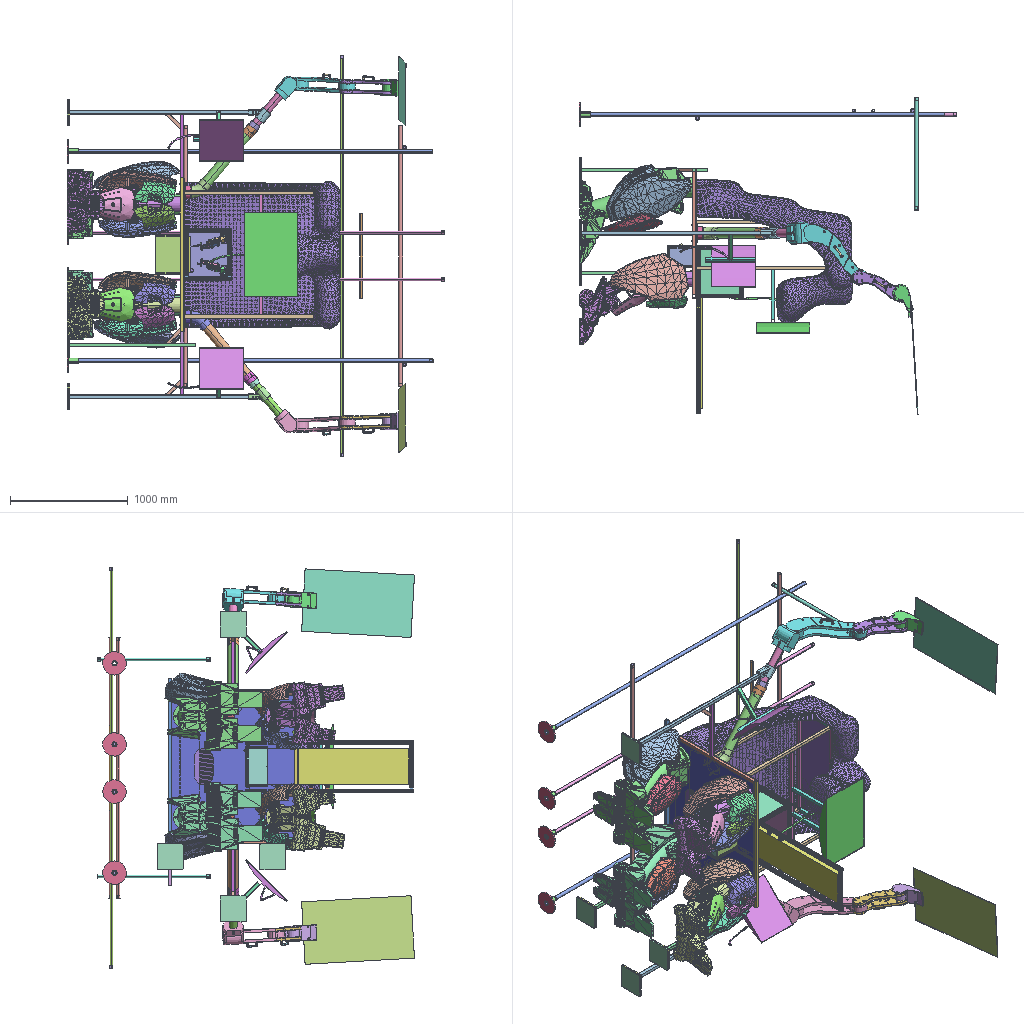Assembly | SolidWorks | 142 different items | 245 placed | box 3202 x 2687 x 3404 mm
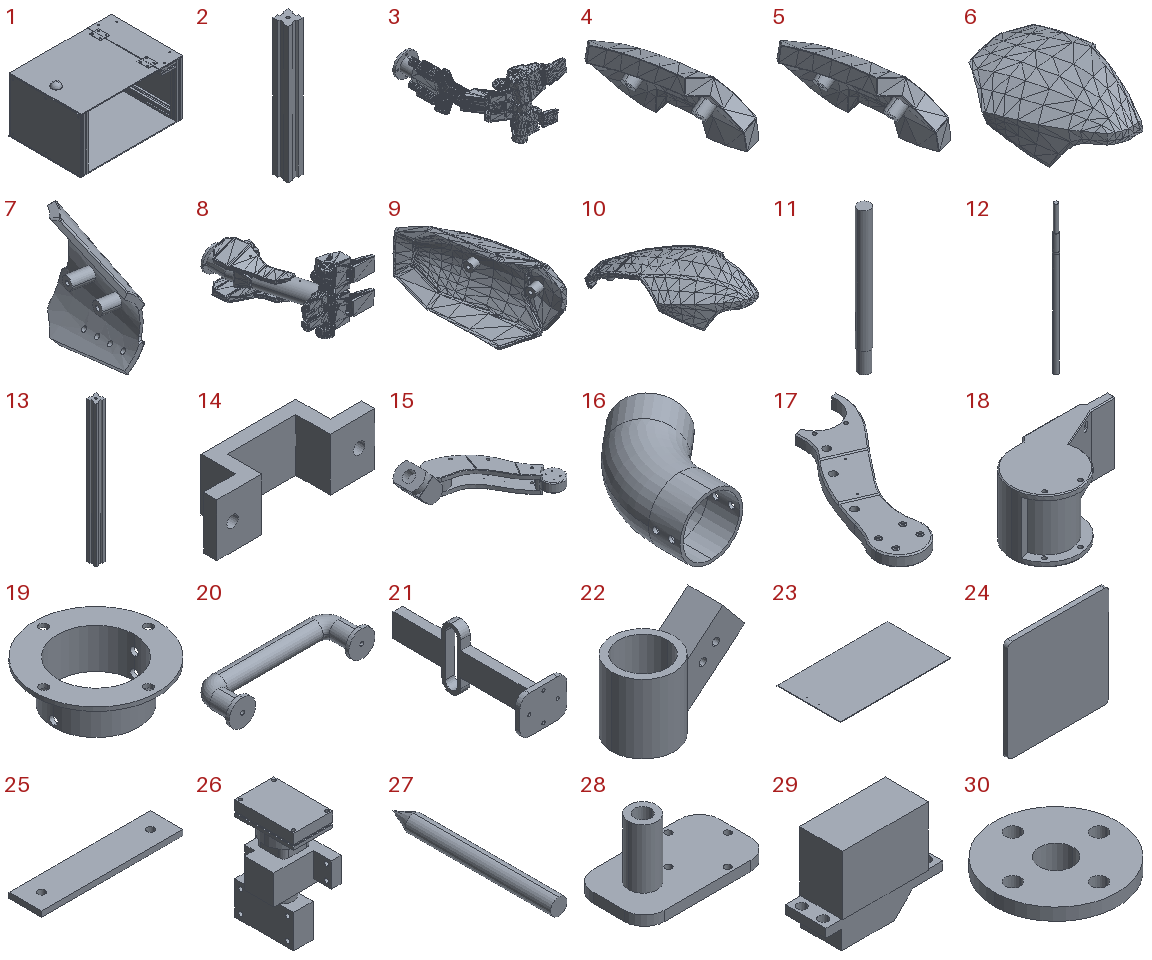Parts list (item | name | quantity | parent item | size | volume | features):
1 | (subassembly) | x1 | - | 346 x 245 x 203 mm | 1584731 mm3 | features CompositeCurve 1
2 | - | x4 | in 1 | 20 x 20 x 180 mm | 60635 mm3 | features CirPattern 1, Extrusion 1, ICE 1
3 | - | x1 | - | - | 34150920 mm3 | features MirrorStock 1
4 | - | x1 | - | 143.42 x 346.686 x 193.978 mm | 2031245 mm3 | features MirrorStock 1
5 | - | x1 | - | 143.42 x 346.686 x 193.978 mm | 2031245 mm3 | features MirrorStock 1
6 | - | x1 | - | 402.328 x 659.123 x 278.681 mm | 8547587 mm3 | features MirrorStock 1
7 | - | x1 | - | 138.848 x 288 x 292.377 mm | 1252657 mm3 | features MirrorStock 1
8 | - | x1 | - | - | 59999692 mm3 | features MirrorStock 1
9 | - | x1 | - | 192.975 x 474.444 x 296.209 mm | 2534423 mm3 | features MirrorStock 1
10 | - | x1 | - | 464.837 x 729.145 x 237.064 mm | 8192368 mm3 | features MirrorStock 1
11 | - | x1 | - | 12 x 12 x 140 mm | 15472 mm3 | features MirrorStock 1
12 | - | x1 | - | 16 x 16 x 460 mm | 67780 mm3 | features MirrorStock 1
13 | - | x1 | in 1 | 20 x 20 x 300 mm | 101058 mm3 | features CirPattern 1, Extrusion 1, ICE 1
14 | - | x1 | - | 60 x 18 x 20 mm | 8448 mm3 | features MirrorStock 1
15 | - | x1 | - | 657.517 x 555 x 192.791 mm | 7755775 mm3 | features MirrorStock 1
16 | - | x1 | - | 167.236 x 220.793 x 100 mm | 316350 mm3 | features MirrorStock 1
17 | - | x2 | - | 271.568 x 416.057 x 25 mm | 864858 mm3 | features MirrorStock 1
18 | - | x1 | - | 270 x 150 x 130 mm | 2349821 mm3 | features MirrorStock 1
19 | - | x1 | - | 160 x 160 x 52 mm | 135135 mm3 | features MirrorStock 1
20 | - | x2 | - | 122 x 37.5 x 22 mm | 26841 mm3 | features MirrorStock 1
21 | - | x1 | - | 50 x 155 x 65 mm | 47254 mm3 | features MirrorStock 1
22 | - | x1 | - | 167.949 x 90.5 x 129.102 mm | 386069 mm3 | features MirrorStock 1
23 | - | x1 | - | 930 x 530 x 5 mm | 2464158 mm3 | features MirrorStock 1
24 | - | x4 | - | 220 x 10 x 220 mm | 483142 mm3 | features Extrusion 1, Fillet 1
25 | - | x1 | - | 130 x 30 x 5 mm | 19158 mm3 | features MirrorStock 1
26 | - | x1 | - | 50 x 78.682 x 114 mm | 167439 mm3 | features MirrorStock 1
27 | - | x1 | - | 8 x 80 x 8 mm | 3686 mm3 | features MirrorStock 1
28 | - | x1 | - | 64 x 36 x 35 mm | 14420 mm3 | features MirrorStock 1
29 | - | x1 | - | 54.44 x 20 x 46.45 mm | 31100 mm3 | features MirrorStock 1
30 | - | x1 | - | 20 x 20 x 4.5 mm | 639.904 mm3 | features MirrorStock 1
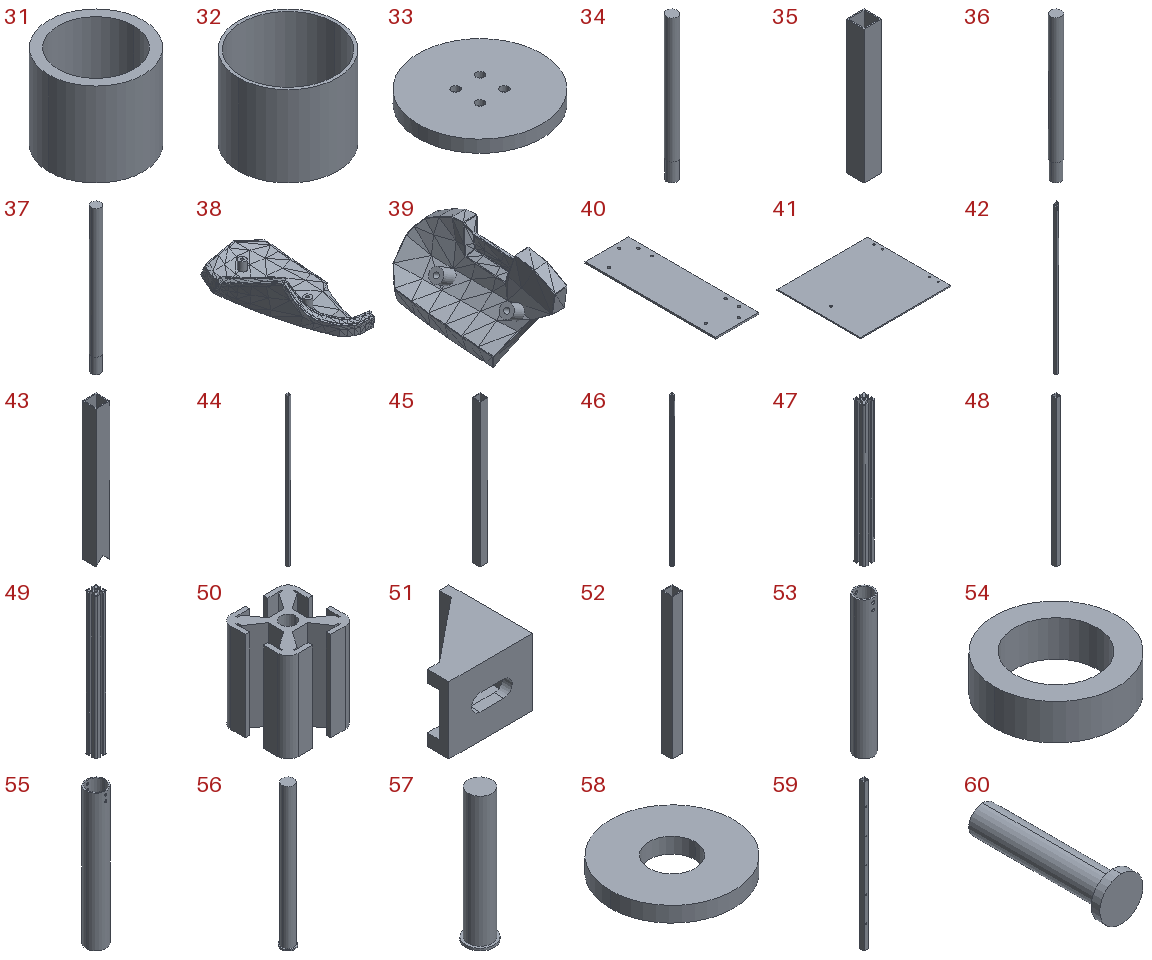31 | - | x1 | - | 90 x 90 x 80 mm | 183218 mm3 | features MirrorStock 1
32 | - | x1 | - | 98 x 98 x 80 mm | 71628 mm3 | features MirrorStock 1
33 | - | x1 | - | 50 x 50 x 20 mm | 10180 mm3 | features MirrorStock 1
34 | - | x1 | - | 12 x 12 x 155 mm | 17169 mm3 | features MirrorStock 1
35 | - | x1 | - | 30 x 30 x 230 mm | 51520 mm3 | features Extrusion 1
36 | - | x4 | - | 12 x 12 x 160 mm | 17734 mm3 | features MirrorStock 1
37 | - | x3 | - | 12 x 12 x 185 mm | 20562 mm3 | features MirrorStock 1
38 | - | x1 | - | 402.328 x 659.123 x 278.681 mm | 8547587 mm3 | features MirrorStock 1
39 | - | x1 | - | 143.42 x 346.686 x 193.978 mm | 2031245 mm3 | features MirrorStock 1
40 | - | x1 | in 1 | 80 x 243 x 3 mm | 57955 mm3 | features Cut 2, Extrusion 1, MirrorPattern 1
41 | - | x1 | in 1 | 263 x 243 x 3 mm | 191442 mm3 | features Cut 2, Extrusion 1, MirrorPattern 1
42 | - | x2 | - | 30 x 30 x 1612 mm | 357438 mm3 | features Cut 1, Extrusion 1, ICE 1
43 | - | x2 | - | 30 x 30 x 300 mm | 66196 mm3 | features Extrusion 1, ICE 1
44 | - | x1 | - | 30 x 30 x 1500 mm | 336000 mm3 | features Extrusion 1
45 | - | x2 | - | 30 x 30 x 540 mm | 120960 mm3 | features Extrusion 1
46 | - | x2 | - | 30 x 30 x 1420 mm | 556341 mm3 | features CirPattern 1, Extrusion 1, Fillet 1, ICE 1
47 | - | x4 | - | 30 x 30 x 367 mm | 143787 mm3 | features CirPattern 1, Extrusion 1, Fillet 1, ICE 1
48 | - | x3 | - | 30 x 30 x 1020 mm | 228480 mm3 | features Extrusion 1
49 | - | x6 | - | 30 x 30 x 380 mm | 148880 mm3 | features CirPattern 1, Extrusion 1, Fillet 1, ICE 1
50 | - | x8 | - | 30 x 30 x 40 mm | 15672 mm3 | features CirPattern 1, Extrusion 1, Fillet 1, ICE 1
51 | - | x2 | - | 35 x 35 x 28 mm | 10804 mm3 | features ICE 3, Extrusion 1, MirrorPattern 1
52 | - | x6 | - | 30 x 30 x 420 mm | 94080 mm3 | features Extrusion 1
53 | - | x1 | - | 70 x 70 x 520 mm | 529289 mm3 | features ICE 4, Cut 1, Extrusion 1
54 | - | x3 | - | 12 x 12 x 3.5 mm | 219.911 mm3 | features Extrusion 1
55 | - | x1 | - | 90 x 90 x 620 mm | 826172 mm3 | features ICE 3, Cut 1, Extrusion 1
56 | - | x2 | - | 12 x 12 x 121 mm | 9538 mm3 | features Extrusion 1, ICE 1
57 | - | x2 | - | 12 x 12 x 56 mm | 4433 mm3 | features Extrusion 1, ICE 1
58 | - | x4 | - | 16 x 16 x 2 mm | 345.575 mm3 | features Extrusion 1
59 | - | x2 | - | 30 x 30 x 1040 mm | 232276 mm3 | features Extrusion 1, ICE 1
60 | - | x2 | - | 12.5 x 40 x 12.5 mm | 2192 mm3 | features Revolution 1
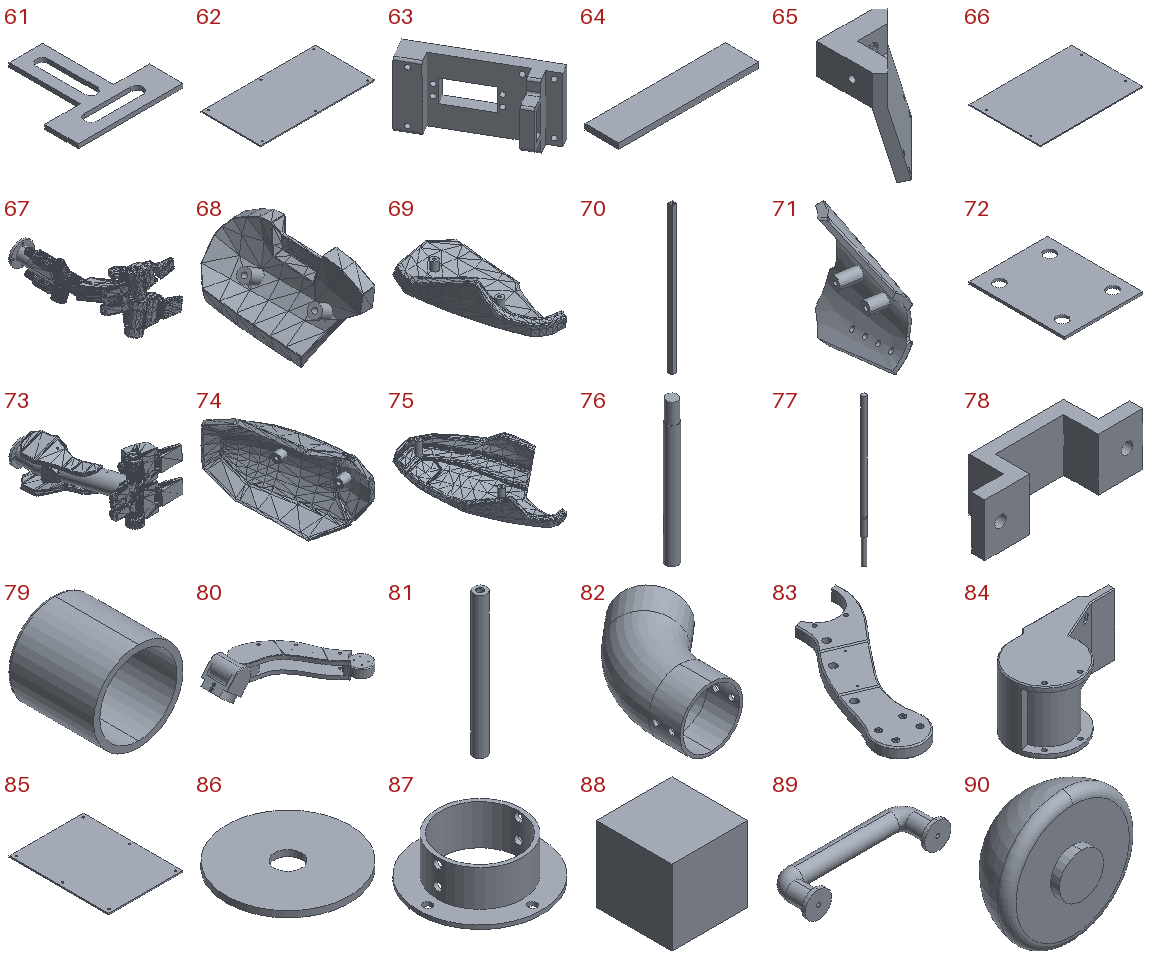61 | - | x1 | - | 50 x 50 x 2 mm | 2035 mm3 | features Extrusion 1
62 | - | x1 | in 1 | 346 x 182 x 3 mm | 188642 mm3 | features Cut 1, Extrusion 1
63 | - | x1 | - | 76.392 x 107.781 x 60 mm | 84689 mm3 | features ICE 7, Fillet 4, Cut 2, Extrusion 1
64 | - | x1 | - | 1250 x 300 x 50 mm | 18750000 mm3 | features Extrusion 1
65 | - | x2 | - | 73.918 x 73.918 x 93.747 mm | 108156 mm3 | features ICE 6, Extrusion 1, MirrorPattern 1
66 | - | x1 | in 1 | 346 x 240 x 3 mm | 248938 mm3 | features Cut 1, Extrusion 1
67 | - | x1 | - | - | 34150920 mm3 | features ICE 11, MirrorPattern 2, BaseBody 1, CirPattern 1, Scale 1
68 | - | x1 | - | 143.42 x 346.686 x 193.978 mm | 2031245 mm3 | features ICE 2, BaseBody 1, Scale 1
69 | - | x1 | - | 402.328 x 659.123 x 278.681 mm | 8547587 mm3 | features ICE 3, BaseBody 1, Scale 1
70 | - | x2 | - | 30 x 30 x 1070 mm | 239680 mm3 | features Extrusion 1
71 | - | x1 | - | 138.848 x 288 x 292.377 mm | 1252666 mm3 | features Fillet 6, ICE 6, MirrorPattern 2, RevCut 1, Revolution 1, Scale 1
72 | - | x2 | in 1 | 31 x 38 x 1 mm | 1114 mm3 | features Extrusion 1
73 | - | x1 | - | - | 59999682 mm3 | features ICE 10, BaseBody 1, Scale 1, Sweep 1
74 | - | x1 | - | 192.975 x 474.444 x 296.209 mm | 2534423 mm3 | features BaseBody 1, ICE 1, Scale 1
75 | - | x1 | - | 464.837 x 729.145 x 237.064 mm | 8192369 mm3 | features ICE 3, BaseBody 1, Scale 1
76 | - | x1 | - | 12 x 12 x 140 mm | 15472 mm3 | features Extrusion 1, ICE 1
77 | - | x1 | - | 16 x 16 x 460 mm | 67780 mm3 | features ICE 2, Extrusion 1
78 | - | x1 | - | 60 x 18 x 20 mm | 8448 mm3 | features Cut 1, Extrusion 1
79 | - | x11 | - | 29 x 28 x 29 mm | 5713 mm3 | features Fillet 1, Revolution 1
80 | - | x1 | - | 657.517 x 555 x 192.791 mm | 7757543 mm3 | features ICE 19, Chamfer 5, Cut 3, Fillet 3, Extrusion 1, MirrorSolid 1
81 | - | x2 | - | 10 x 10 x 110 mm | 8282 mm3 | features 3DProfileFeature 1, Extrusion 1, HoleWzd 1, MirrorPattern 1
82 | - | x1 | - | 167.236 x 220.793 x 100 mm | 316350 mm3 | features ICE 1, MirrorPattern 1, Sweep 1
83 | - | x2 | - | 271.568 x 416.057 x 25 mm | 865403 mm3 | features ICE 8, Cut 3, Chamfer 2, Fillet 2, MirrorPattern 2, Extrusion 1, Scale 1
84 | - | x1 | - | 270 x 150 x 130 mm | 2349821 mm3 | features ICE 4, Cut 2, Chamfer 1, Extrusion 1, MirrorSolid 1
85 | - | x2 | in 1 | 178 x 240 x 3 mm | 127886 mm3 | features Cut 1, Extrusion 1
86 | - | x4 | - | 200 x 200 x 10 mm | 299298 mm3 | features Extrusion 1
87 | - | x1 | - | 160 x 160 x 52 mm | 135135 mm3 | features ICE 4, CirPattern 1, Extrusion 1
88 | - | x1 | - | 80 x 80 x 80 mm | 512000 mm3 | features Extrusion 1
89 | - | x2 | - | 122 x 37.5 x 22 mm | 26841 mm3 | features ICE 3, Sweep 1
90 | - | x1 | in 1 | 29.69 x 17 x 29.69 mm | 7127 mm3 | features Fillet 1, ICE 1, Revolution 1
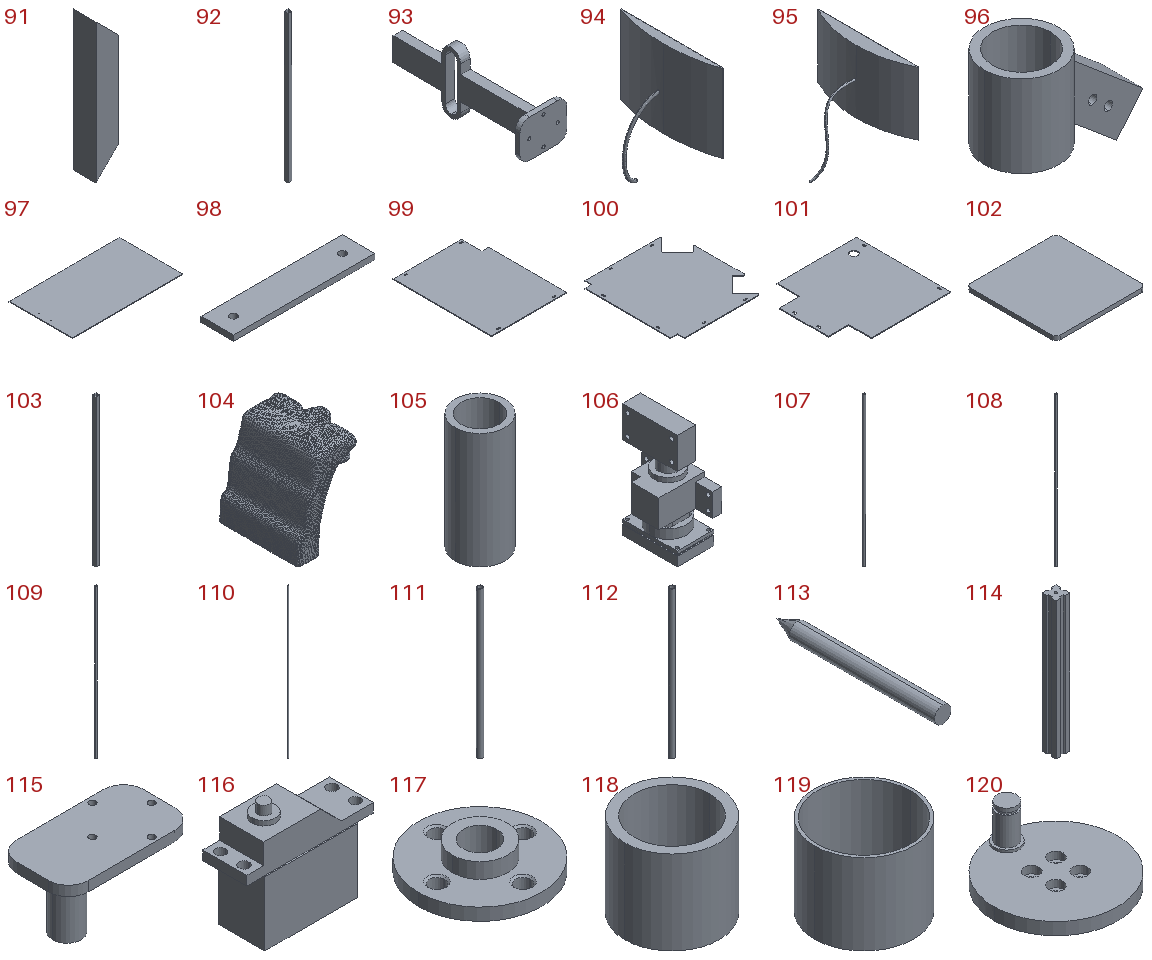91 | - | x4 | - | 30 x 30 x 185 mm | 34720 mm3 | features Extrusion 1, ICE 1
92 | - | x4 | - | 30 x 30 x 1112 mm | 249088 mm3 | features Extrusion 1
93 | - | x1 | - | 50 x 155 x 65 mm | 47254 mm3 | features ICE 3, Cut 1, Extrusion 1, Fillet 1
94 | - | x2 | - | 155.98 x 493 x 640.45 mm | 5277382 mm3 | features 3DProfileFeature 2, Extrusion 1, ICE 1, Sweep 1
95 | - | x1 | - | 360.915 x 719 x 753.544 mm | 19467710 mm3 | features 3DProfileFeature 2, Extrusion 1, ICE 1, Sweep 1
96 | - | x1 | - | 167.949 x 90.5 x 129.102 mm | 386069 mm3 | features ICE 3, Extrusion 1, MirrorPattern 1
97 | - | x1 | - | 930 x 530 x 5 mm | 2464158 mm3 | features Cut 1, Extrusion 1
98 | - | x1 | - | 130 x 30 x 5 mm | 19158 mm3 | features Extrusion 1
99 | - | x2 | - | 333 x 436 x 3 mm | 426578 mm3 | features Cut 2, Extrusion 1
100 | - | x1 | - | 404 x 436 x 3 mm | 471052 mm3 | features ICE 3, Cut 2, Extrusion 1, Fillet 1, MirrorPattern 1
101 | - | x1 | - | 393 x 372 x 3 mm | 392382 mm3 | features Cut 2, ICE 2, Extrusion 1
102 | - | x4 | - | 220 x 220 x 10 mm | 483142 mm3 | features Extrusion 1, Fillet 1
103 | - | x1 | - | 30 x 30 x 1300 mm | 291200 mm3 | features Extrusion 1
104 | - | x1 | - | - | 395223712 mm3 | features BaseBody 1, ICE 1, Scale 1
105 | - | x4 | - | 43 x 43 x 100 mm | 59690 mm3 | features Extrusion 1
106 | - | x1 | - | 50 x 78.682 x 114 mm | 167439 mm3 | features ICE 9, Cut 3, Extrusion 1
107 | - | x2 | - | 32 x 32 x 2210 mm | 416575 mm3 | features Extrusion 1
108 | - | x2 | - | 32 x 32 x 3100 mm | 584336 mm3 | features Extrusion 1
109 | - | x2 | - | 32 x 32 x 3200 mm | 603186 mm3 | features Extrusion 1
110 | - | x1 | - | 25 x 25 x 3400 mm | 491345 mm3 | features Extrusion 1
111 | - | x1 | - | 25 x 25 x 720 mm | 104050 mm3 | features Extrusion 1
112 | - | x2 | - | 32 x 32 x 950 mm | 179071 mm3 | features Extrusion 1
113 | - | x1 | - | 8 x 80 x 8 mm | 3686 mm3 | features Revolution 1
114 | - | x4 | in 1 | 20 x 20 x 202 mm | 68046 mm3 | features CirPattern 1, Extrusion 1, ICE 1
115 | - | x1 | - | 64 x 36 x 35 mm | 14420 mm3 | features ICE 6, CirPattern 1, Extrusion 1, Fillet 1
116 | - | x1 | - | 54.44 x 20 x 46.45 mm | 31100 mm3 | features ICE 5, Chamfer 1, Extrusion 1
117 | - | x1 | - | 20 x 20 x 4.5 mm | 639.904 mm3 | features ICE 2, 3DProfileFeature 1, CirPattern 1, Extrusion 1, HoleWzd 1
118 | - | x1 | - | 90 x 90 x 80 mm | 183218 mm3 | features Extrusion 1
119 | - | x1 | - | 98 x 98 x 80 mm | 71628 mm3 | features Extrusion 1
120 | - | x1 | - | 50 x 50 x 20 mm | 10180 mm3 | features ICE 5, CirPattern 1, Extrusion 1
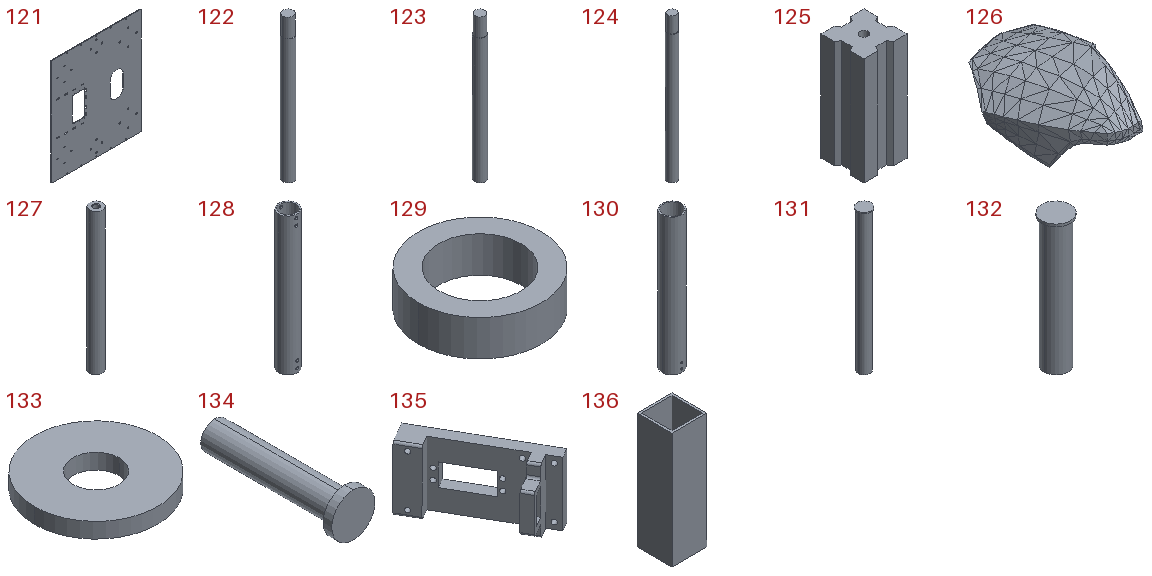121 | - | x1 | - | 1096 x 5 x 1296 mm | 6599670 mm3 | features Cut 7, MirrorPattern 4, LPattern 3, Fillet 2, ICE 2, Extrusion 1
122 | - | x1 | - | 12 x 12 x 155 mm | 17169 mm3 | features Extrusion 1, ICE 1
123 | - | x4 | - | 12 x 12 x 160 mm | 17734 mm3 | features Extrusion 1, ICE 1
124 | - | x3 | - | 12 x 12 x 185 mm | 20562 mm3 | features Extrusion 1, ICE 1
125 | - | x1 | in 1 | 20 x 20 x 50 mm | 16843 mm3 | features CirPattern 1, Extrusion 1, ICE 1
126 | - | x1 | - | 402.328 x 659.123 x 278.681 mm | 8547587 mm3 | features MirrorStock 1
127 | - | x2 | - | 10 x 10 x 110 mm | 8282 mm3 | features MirrorStock 1
128 | - | x1 | - | 70 x 70 x 520 mm | 527553 mm3 | features MirrorStock 1
129 | - | x3 | - | 12 x 12 x 3.5 mm | 219.911 mm3 | features MirrorStock 1
130 | - | x1 | - | 90 x 90 x 620 mm | 826173 mm3 | features MirrorStock 1
131 | - | x1 | - | 12 x 12 x 121 mm | 9538 mm3 | features MirrorStock 1
132 | - | x2 | - | 12 x 12 x 56 mm | 4433 mm3 | features MirrorStock 1
133 | - | x4 | - | 16 x 16 x 2 mm | 345.575 mm3 | features MirrorStock 1
134 | - | x2 | - | 12.5 x 40 x 12.5 mm | 2192 mm3 | features MirrorStock 1
135 | - | x1 | - | 76.392 x 107.781 x 60 mm | 84689 mm3 | features MirrorStock 1
136 | - | x1 | - | 30 x 30 x 100 mm | 22400 mm3 | features Extrusion 1
137 | circlips for shaft--type a small gb | x1 | - | - | - | -
138 | hex bolts with split pin hole-grade ab gb | x1 | - | - | - | -
139 | hex nuts, style 1-grades ab gb | x1 | - | - | - | -
140 | hexagon nuts grade c gb | x1 | - | - | - | -
141 | hexagon socket head cap screws gb | x1 | - | - | - | -
142 | slotted pan head screws gb | x1 | - | - | - | -
Mates (type | each side: item.copy, entity, surface, feature):
In the top assembly
Coincident | 59.1 face plane Boss-Extrude 1 | 121.1 face plane Boss-Extrude 1
DistanceDim | 59.1 face plane Boss-Extrude 1 | 121.1 face plane Boss-Extrude 1
Symmetric | 121.1 plane | 52.1 face plane Boss-Extrude 1 | 52.2 face plane Boss-Extrude 1
Symmetric | 47.1 face plane Boss-Extrude 1 | 47.2 face plane Boss-Extrude 1 | 64.1 plane
Coincident | assembly face | assembly face | 2 times
Coincident | assembly face | 35.1 face plane Boss-Extrude 1 | 2 times
Coincident | 121.1 face plane Boss-Extrude 1 | 59.2 face plane Boss-Extrude 1
Coincident | 121.1 face plane Boss-Extrude 1 | 46.1 face plane Boss-Extrude 1
Coincident | 50.1 face plane Boss-Extrude 1 | 64.1 face plane Boss-Extrude 1
Coincident | 121.1 face plane Boss-Extrude 1 | 92.1 face plane Boss-Extrude 1
Coincident | 64.1 face plane Boss-Extrude 1 | 51.1 face plane Boss-Extrude 1
DistanceDim | 121.1 face plane Boss-Extrude 1 | 59.2 face plane Boss-Extrude 1
Coincident | 65.1 face plane Boss-Extrude 2 | 106.1 face plane Boss-Extrude 6
Symmetric | 65.1 plane | 106.1 face plane Boss-Extrude 1 | 106.1 face plane Boss-Extrude 1
Coincident | 63.1 face plane Boss-Extrude 2 | assembly face
Concentric | 63.1 face cylinder Cut-Extrude 6 | assembly face
DistanceDim | 106.1 face plane Boss-Extrude 6 | 65.1 face plane Boss-Extrude 2
Concentric | 63.1 face cylinder Cut-Extrude 6 | 106.1 face cylinder Cut-Extrude 3 | 2 times
Coincident | 63.1 edge | 106.1 face plane Boss-Extrude 10
Coincident | 121.1 face plane Boss-Extrude 1 | 44.1 face plane Boss-Extrude 1
Coincident | 59.1 face plane Boss-Extrude 1 | 44.1 face plane Boss-Extrude 1
Symmetric | 121.1 plane | 44.1 face plane Boss-Extrude 1 | 44.1 face plane Boss-Extrude 1
Coincident | assembly face | 44.1 face plane Boss-Extrude 1 | 2 times
Coincident | 35.1 face plane Boss-Extrude 1 | 44.1 face plane Boss-Extrude 1
Concentric | 121.1 face cylinder Cut-Extrude 4 | 73.1 face cylinder Boss-Extrude 4 | 2 times
Coincident | 121.1 face plane Boss-Extrude 1 | 73.1 face plane Boss-Extrude 4
Coincident | 121.1 face plane Boss-Extrude 1 | 67.1 face plane Boss-Extrude 1
Concentric | 121.1 face cylinder Cut-Extrude 5 | 67.1 face cylinder CirPattern 1
Concentric | 121.1 face cylinder Cut-Extrude 5 | 67.1 face cylinder Cut-Extrude 2
DistanceDim | 49.1 face plane Boss-Extrude 1 | 64.1 face plane Boss-Extrude 1
Coincident | 59.2 face plane Boss-Extrude 1 | 103.1 face plane Boss-Extrude 1 | 2 times
Coincident | 121.1 face plane Boss-Extrude 1 | 103.1 face plane Boss-Extrude 1
Coincident | assembly face | 136.1 face plane Boss-Extrude 1 | 2 times
Coincident | 59.2 face plane Boss-Extrude 1 | 136.1 face plane Boss-Extrude 1 | 2 times
DistanceDim | 136.1 face plane Boss-Extrude 1 | 103.1 face plane Boss-Extrude 1
Coincident | 136.1 face plane Boss-Extrude 1 | 70.1 face plane Boss-Extrude 1 | 2 times
Coincident | 35.1 face plane Boss-Extrude 1 | 70.2 face plane Boss-Extrude 1 | 2 times
Coincident | 44.1 face plane Boss-Extrude 1 | 70.2 face plane Boss-Extrude 1 | 2 times
Coincident | 102.1 face plane Boss-Extrude 1 | 102.2 face plane Boss-Extrude 1
DistanceDim | 59.2 face plane Boss-Extrude 1 | 24.1 face plane Boss-Extrude 1
DistanceDim | 121.1 face plane Boss-Extrude 1 | 103.1 face plane Boss-Extrude 1
Coincident | 45.1 face plane Boss-Extrude 1 | 59.1 face plane Boss-Extrude 1 | 2 times
Coincident | 121.1 face plane Boss-Extrude 1 | 2.1 face plane Boss-Extrude 1
Symmetric | 121.1 plane | 47.2 face plane Boss-Extrude 1 | 47.1 face plane Boss-Extrude 1
Coincident | 121.1 face plane Boss-Extrude 1 | 47.2 face plane Boss-Extrude 1
Coincident | 121.1 face plane Cut-Extrude 6 | 2.2 face plane Boss-Extrude 1
Coincident | 121.1 face plane Cut-Extrude 6 | 66.1 face plane Boss-Extrude 1
Coincident | 42.1 face plane Boss-Extrude 1 | 43.1 face plane Cut-Extrude 1 | 2 times
DistanceDim | 45.1 face plane Boss-Extrude 1 | 44.1 face plane Boss-Extrude 1
Coincident | 43.1 face plane Boss-Extrude 1 | 52.3 face plane Boss-Extrude 1 | 2 times
Coincident | 59.1 face plane Boss-Extrude 1 | 103.1 face plane Boss-Extrude 1
DistanceDim | 94.1 face plane Cut-Extrude 1 | 52.3 face plane Boss-Extrude 1
Coincident | 94.1 face plane Boss-Extrude 1 | 52.3 face plane Boss-Extrude 1
Coincident | 70.1 face plane Boss-Extrude 1 | 91.1 face plane Cut-Extrude 1
Coincident | 70.1 face plane Boss-Extrude 1 | 91.1 face plane Boss-Extrude 1
Coincident | 136.1 face plane Boss-Extrude 1 | 91.1 face plane Cut-Extrude 1
Coincident | 70.2 face plane Boss-Extrude 1 | 91.2 face plane Boss-Extrude 1
Coincident | 35.1 face plane Boss-Extrude 1 | 91.2 face plane Cut-Extrude 1
Coincident | 70.2 face plane Boss-Extrude 1 | 91.2 face plane Cut-Extrude 1
Coincident | 45.1 face plane Boss-Extrude 1 | 91.3 face plane Cut-Extrude 1
Coincident | 42.1 face plane Boss-Extrude 1 | 91.3 face plane Cut-Extrude 1
Coincident | 42.1 face plane Boss-Extrude 1 | 91.3 edge
Symmetric | 43.1 face plane Boss-Extrude 1 | 43.1 face plane Boss-Extrude 1 | 52.3 plane
Coincident | 86.1 face plane Boss-Extrude 1 | 102.3 face plane Boss-Extrude 1
Parallel | 107.1 plane | 70.2 face plane Boss-Extrude 1
Coincident | 121.1 face plane Boss-Extrude 1 | 87.1 face plane Boss-Extrude 1
Concentric | 121.1 select_type:24 | 87.1 face cylinder CirPattern 1 | 2 times
Concentric | 87.1 face cylinder Cut-Extrude 3 | 56.1 face cylinder Boss-Extrude 1
Tangent | 87.1 face cylinder Boss-Extrude 1 | 56.1 face plane Boss-Extrude 2
Parallel | 42.1 face plane Boss-Extrude 1 | 96.1 face plane Mirror 1
Coincident | 56.1 face plane Boss-Extrude 2 | 56.2 face plane Boss-Extrude 2
In subassembly 1
Coincident | 2.3 face plane Boss-Extrude 1 | 2.4 face plane Boss-Extrude 1 | 2 times
Coincident | 2.4 face plane Boss-Extrude 1 | 85.1 face plane Boss-Extrude 1
DistanceDim | 2.4 face plane Boss-Extrude 1 | 85.1 face plane Boss-Extrude 1
DistanceDim | 2.3 face plane Boss-Extrude 1 | 85.1 face plane Boss-Extrude 1
Coincident | 2.3 face plane Boss-Extrude 1 | 66.2 face plane Boss-Extrude 1
Coincident | 2.5 face plane Boss-Extrude 1 | 66.2 face plane Boss-Extrude 1
Coincident | 2.6 face plane Boss-Extrude 1 | 66.2 face plane Boss-Extrude 1
DistanceDim | 85.1 face plane Boss-Extrude 1 | 2.4 face plane Boss-Extrude 1
Coincident | 2.3 face plane Boss-Extrude 1 | 2.6 face plane Boss-Extrude 1
Coincident | 2.5 face plane Boss-Extrude 1 | 2.6 face plane Boss-Extrude 1
Coincident | 2.4 face plane Boss-Extrude 1 | 2.5 face plane Boss-Extrude 1
Coincident | 2.6 face plane Boss-Extrude 1 | 85.2 face plane Boss-Extrude 1
Coincident | 85.1 face plane Boss-Extrude 1 | 85.2 face plane Boss-Extrude 1 | 2 times
Coincident | 85.1 face plane Boss-Extrude 1 | 66.2 face plane Boss-Extrude 1
Coincident | 66.2 face plane Boss-Extrude 1 | 85.2 face plane Boss-Extrude 1 | 2 times
Coincident | 2.5 face plane Boss-Extrude 1 | 62.1 face plane Boss-Extrude 1
Coincident | 66.2 face plane Boss-Extrude 1 | 62.1 face plane Boss-Extrude 1
Coincident | 85.2 face plane Boss-Extrude 1 | 62.1 face plane Boss-Extrude 1
Coincident | 66.2 face plane Boss-Extrude 1 | 114.1 face plane Boss-Extrude 1
Coincident | 2.3 face plane Boss-Extrude 1 | 114.1 face plane Boss-Extrude 1
Coincident | 2.4 face plane Boss-Extrude 1 | 114.1 face plane Boss-Extrude 1
Coincident | 114.1 face plane Boss-Extrude 1 | 114.2 face plane Boss-Extrude 1
Coincident | 85.2 face plane Boss-Extrude 1 | 114.2 face plane Boss-Extrude 1
Coincident | 2.6 face plane Boss-Extrude 1 | 114.2 face plane Boss-Extrude 1
Coincident | 2.6 face plane Boss-Extrude 1 | 114.3 face plane Boss-Extrude 1 | 2 times
Coincident | 85.2 face plane Boss-Extrude 1 | 114.3 face plane Boss-Extrude 1
Coincident | 2.3 face plane Boss-Extrude 1 | 114.4 face plane Boss-Extrude 1 | 3 times
Coincident | 2.6 face plane Boss-Extrude 1 | 40.1 face plane Boss-Extrude 1
Coincident | 85.2 face plane Boss-Extrude 1 | 40.1 face plane Boss-Extrude 1 | 2 times
Coincident | 40.1 face plane Boss-Extrude 1 | 13.1 face plane Boss-Extrude 1
Coincident | 2.5 face plane Boss-Extrude 1 | 13.1 face plane Boss-Extrude 1
Coincident | 2.4 face plane Boss-Extrude 1 | 13.1 face plane Boss-Extrude 1
Coincident | 40.1 face plane Boss-Extrude 1 | 72.1 face plane Boss-Extrude 1
Concentric | 40.1 face cylinder Cut-Extrude 2 | 72.1 face cylinder Boss-Extrude 1
Concentric | 40.1 edge | 72.1 face cylinder Boss-Extrude 1
Coincident | 40.1 face plane Boss-Extrude 1 | 72.2 face plane Boss-Extrude 1
Concentric | 40.1 face cylinder Mirror 1 | 72.2 face cylinder Boss-Extrude 1 | 2 times
Concentric | 72.2 face cylinder Boss-Extrude 1 | 41.1 face cylinder Mirror 1 | 2 times
Coincident | 72.2 face plane Boss-Extrude 1 | 41.1 face plane Boss-Extrude 1
Coincident | 2.6 face plane Boss-Extrude 1 | 125.1 face plane Boss-Extrude 1 | 2 times
Coincident | 40.1 face plane Boss-Extrude 1 | 125.1 face plane Boss-Extrude 1
Concentric | 41.1 face cylinder Cut-Extrude 3 | 90.1 face cylinder Boss-Extrude 1
Coincident | 41.1 face plane Boss-Extrude 1 | 90.1 face plane Boss-Extrude 1